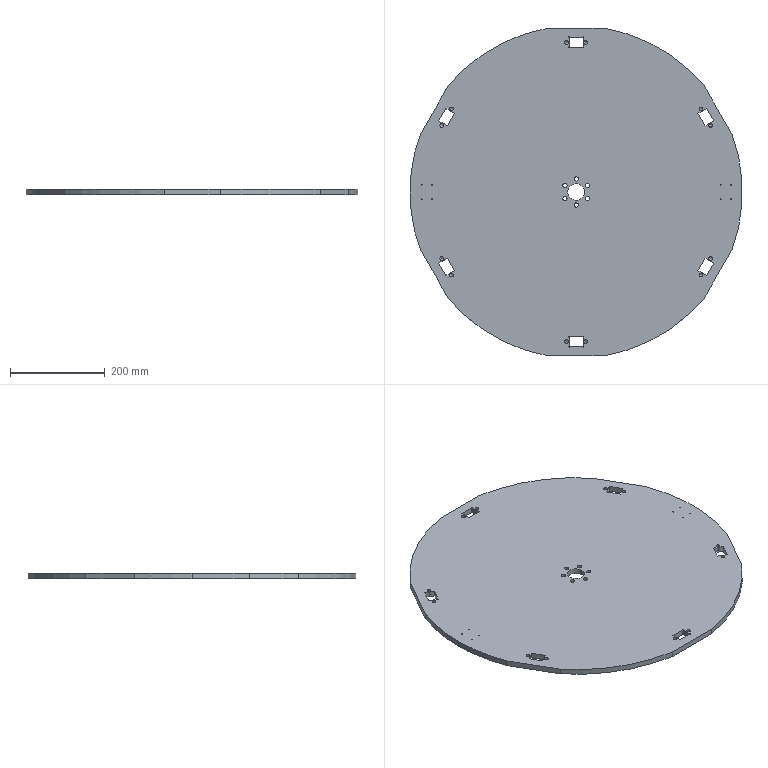Part | SolidWorks | features CirPattern 5, ICE 3, HoleWzd 2, Extrusion 1 | 1 solid | 141 faces | box 700 x 690 x 12 mm | volume 4521944 mm3 | cylinder 69 | plane 48 | cone 24 | commonest cylinder face diameters 2 x24 8.2 x24 9 x12 700 x7 35.5 x2